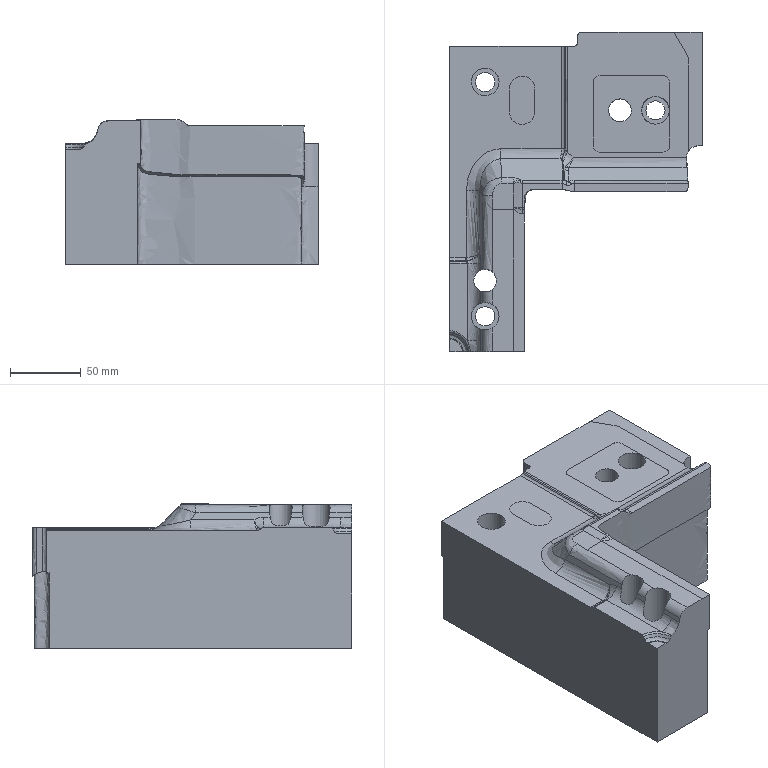Part | NX | features solid 2 | 1 solid | 103 faces | box 178 x 225.007 x 101.792 mm | volume 2018224 mm3 | spline 86 | plane 9 | cylinder 8 | commonest cylinder face diameters 13.5 x3 19.5 x3 16 x2